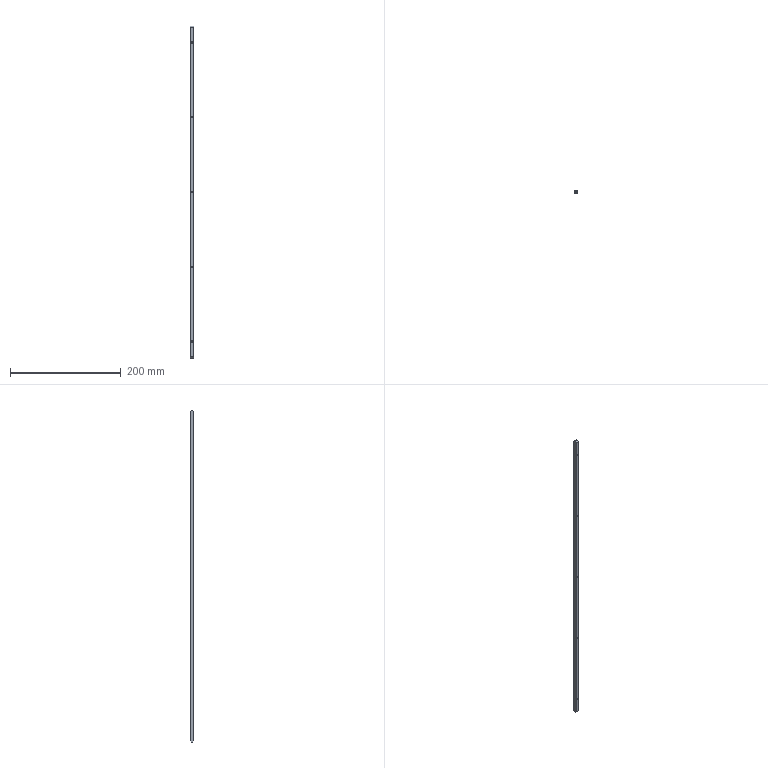Part | SolidWorks | features 3DProfileFeature 1, Chamfer 1, Extrusion 1, HoleWzd 1 | 1 solid | 20 faces | box 6 x 6 x 600 mm | volume 21405 mm3 | cylinder 10 | plane 10 | commonest cylinder face diameters 2.5 x10
STEP:
#1=CARTESIAN_POINT('',(0.,-3.,163.75));
#2=VERTEX_POINT('',#1);
#3=CARTESIAN_POINT('',(0.,-3.,166.25));
#4=VERTEX_POINT('',#3);
#5=CARTESIAN_POINT('',(0.,-3.,165.));
#6=DIRECTION('',(0.,1.,0.));
#7=DIRECTION('',(0.,0.,1.));
#8=AXIS2_PLACEMENT_3D('',#5,#6,#7);
#9=CIRCLE('',#8,1.25);
#10=EDGE_CURVE('',#2,#4,#9,.T.);
#11=ORIENTED_EDGE('',*,*,#10,.F.);
#12=CARTESIAN_POINT('',(0.,3.,163.75));
#13=VERTEX_POINT('',#12);
#14=CARTESIAN_POINT('',(0.,3.,163.75));
#15=DIRECTION('',(0.,1.,0.));
#16=VECTOR('',#15,1000.);
#17=LINE('',#14,#16);
#18=EDGE_CURVE('',#2,#13,#17,.T.);
#19=ORIENTED_EDGE('',*,*,#18,.T.);
#20=CARTESIAN_POINT('',(0.,3.,166.25));
#21=VERTEX_POINT('',#20);
#22=CARTESIAN_POINT('',(0.,3.,165.));
#23=DIRECTION('',(0.,1.,0.));
#24=DIRECTION('',(0.,0.,1.));
#25=AXIS2_PLACEMENT_3D('',#22,#23,#24);
#26=CIRCLE('',#25,1.25);
#27=EDGE_CURVE('',#13,#21,#26,.T.);
#28=ORIENTED_EDGE('',*,*,#27,.T.);
#29=CARTESIAN_POINT('',(0.,3.,166.25));
#30=DIRECTION('',(0.,1.,0.));
#31=VECTOR('',#30,1000.);
#32=LINE('',#29,#31);
#33=EDGE_CURVE('',#4,#21,#32,.T.);
#34=ORIENTED_EDGE('',*,*,#33,.F.);
#35=EDGE_LOOP('',(#11,#19,#28,#34));
#36=FACE_OUTER_BOUND('',#35,.T.);
#37=CARTESIAN_POINT('',(0.,3.,165.));
#38=DIRECTION('',(0.,1.,0.));
#39=DIRECTION('',(0.,0.,1.));
#40=AXIS2_PLACEMENT_3D('',#37,#38,#39);
#41=CYLINDRICAL_SURFACE('',#40,1.25);
#42=ADVANCED_FACE('',(#36),#41,.F.);
#43=CARTESIAN_POINT('',(0.,-3.,298.75));
#44=VERTEX_POINT('',#43);
#45=CARTESIAN_POINT('',(0.,-3.,301.25));
#46=VERTEX_POINT('',#45);
#47=CARTESIAN_POINT('',(0.,-3.,300.));
#48=DIRECTION('',(0.,1.,0.));
#49=DIRECTION('',(0.,0.,1.));
#50=AXIS2_PLACEMENT_3D('',#47,#48,#49);
#51=CIRCLE('',#50,1.25);
#52=EDGE_CURVE('',#44,#46,#51,.T.);
#53=ORIENTED_EDGE('',*,*,#52,.F.);
#54=CARTESIAN_POINT('',(0.,3.,298.75));
#55=VERTEX_POINT('',#54);
#56=CARTESIAN_POINT('',(0.,3.,298.75));
#57=DIRECTION('',(0.,1.,0.));
#58=VECTOR('',#57,1000.);
#59=LINE('',#56,#58);
#60=EDGE_CURVE('',#44,#55,#59,.T.);
#61=ORIENTED_EDGE('',*,*,#60,.T.);
#62=CARTESIAN_POINT('',(0.,3.,301.25));
#63=VERTEX_POINT('',#62);
#64=CARTESIAN_POINT('',(0.,3.,300.));
#65=DIRECTION('',(0.,1.,0.));
#66=DIRECTION('',(0.,0.,1.));
#67=AXIS2_PLACEMENT_3D('',#64,#65,#66);
#68=CIRCLE('',#67,1.25);
#69=EDGE_CURVE('',#55,#63,#68,.T.);
#70=ORIENTED_EDGE('',*,*,#69,.T.);
#71=CARTESIAN_POINT('',(0.,3.,301.25));
#72=DIRECTION('',(0.,1.,0.));
#73=VECTOR('',#72,1000.);
#74=LINE('',#71,#73);
#75=EDGE_CURVE('',#46,#63,#74,.T.);
#76=ORIENTED_EDGE('',*,*,#75,.F.);
#77=EDGE_LOOP('',(#53,#61,#70,#76));
#78=FACE_OUTER_BOUND('',#77,.T.);
#79=CARTESIAN_POINT('',(0.,3.,300.));
#80=DIRECTION('',(0.,1.,0.));
#81=DIRECTION('',(0.,0.,1.));
#82=AXIS2_PLACEMENT_3D('',#79,#80,#81);
#83=CYLINDRICAL_SURFACE('',#82,1.25);
#84=ADVANCED_FACE('',(#78),#83,.F.);
#85=CARTESIAN_POINT('',(0.,-3.,433.75));
#86=VERTEX_POINT('',#85);
#87=CARTESIAN_POINT('',(0.,-3.,436.25));
#88=VERTEX_POINT('',#87);
#89=CARTESIAN_POINT('',(0.,-3.,435.));
#90=DIRECTION('',(0.,1.,0.));
#91=DIRECTION('',(0.,0.,1.));
#92=AXIS2_PLACEMENT_3D('',#89,#90,#91);
#93=CIRCLE('',#92,1.25);
#94=EDGE_CURVE('',#86,#88,#93,.T.);
#95=ORIENTED_EDGE('',*,*,#94,.F.);
#96=CARTESIAN_POINT('',(0.,3.,433.75));
#97=VERTEX_POINT('',#96);
#98=CARTESIAN_POINT('',(0.,3.,433.75));
#99=DIRECTION('',(0.,1.,0.));
#100=VECTOR('',#99,1000.);
#101=LINE('',#98,#100);
#102=EDGE_CURVE('',#86,#97,#101,.T.);
#103=ORIENTED_EDGE('',*,*,#102,.T.);
#104=CARTESIAN_POINT('',(0.,3.,436.25));
#105=VERTEX_POINT('',#104);
#106=CARTESIAN_POINT('',(0.,3.,435.));
#107=DIRECTION('',(0.,1.,0.));
#108=DIRECTION('',(0.,0.,1.));
#109=AXIS2_PLACEMENT_3D('',#106,#107,#108);
#110=CIRCLE('',#109,1.25);
#111=EDGE_CURVE('',#97,#105,#110,.T.);
#112=ORIENTED_EDGE('',*,*,#111,.T.);
#113=CARTESIAN_POINT('',(0.,3.,436.25));
#114=DIRECTION('',(0.,1.,0.));
#115=VECTOR('',#114,1000.);
#116=LINE('',#113,#115);
#117=EDGE_CURVE('',#88,#105,#116,.T.);
#118=ORIENTED_EDGE('',*,*,#117,.F.);
#119=EDGE_LOOP('',(#95,#103,#112,#118));
#120=FACE_OUTER_BOUND('',#119,.T.);
#121=CARTESIAN_POINT('',(0.,3.,435.));
#122=DIRECTION('',(0.,1.,0.));
#123=DIRECTION('',(0.,0.,1.));
#124=AXIS2_PLACEMENT_3D('',#121,#122,#123);
#125=CYLINDRICAL_SURFACE('',#124,1.25);
#126=ADVANCED_FACE('',(#120),#125,.F.);
#127=CARTESIAN_POINT('',(0.,-3.,568.75));
#128=VERTEX_POINT('',#127);
#129=CARTESIAN_POINT('',(0.,-3.,571.25));
#130=VERTEX_POINT('',#129);
#131=CARTESIAN_POINT('',(0.,-3.,570.));
#132=DIRECTION('',(0.,1.,0.));
#133=DIRECTION('',(0.,0.,1.));
#134=AXIS2_PLACEMENT_3D('',#131,#132,#133);
#135=CIRCLE('',#134,1.25);
#136=EDGE_CURVE('',#128,#130,#135,.T.);
#137=ORIENTED_EDGE('',*,*,#136,.F.);
#138=CARTESIAN_POINT('',(0.,3.,568.75));
#139=VERTEX_POINT('',#138);
#140=CARTESIAN_POINT('',(0.,3.,568.75));
#141=DIRECTION('',(0.,1.,0.));
#142=VECTOR('',#141,1000.);
#143=LINE('',#140,#142);
#144=EDGE_CURVE('',#128,#139,#143,.T.);
#145=ORIENTED_EDGE('',*,*,#144,.T.);
#146=CARTESIAN_POINT('',(0.,3.,571.25));
#147=VERTEX_POINT('',#146);
#148=CARTESIAN_POINT('',(0.,3.,570.));
#149=DIRECTION('',(0.,1.,0.));
#150=DIRECTION('',(0.,0.,1.));
#151=AXIS2_PLACEMENT_3D('',#148,#149,#150);
#152=CIRCLE('',#151,1.25);
#153=EDGE_CURVE('',#139,#147,#152,.T.);
#154=ORIENTED_EDGE('',*,*,#153,.T.);
#155=CARTESIAN_POINT('',(0.,3.,571.25));
#156=DIRECTION('',(0.,1.,0.));
#157=VECTOR('',#156,1000.);
#158=LINE('',#155,#157);
#159=EDGE_CURVE('',#130,#147,#158,.T.);
#160=ORIENTED_EDGE('',*,*,#159,.F.);
#161=EDGE_LOOP('',(#137,#145,#154,#160));
#162=FACE_OUTER_BOUND('',#161,.T.);
#163=CARTESIAN_POINT('',(0.,3.,570.));
#164=DIRECTION('',(0.,1.,0.));
#165=DIRECTION('',(0.,0.,1.));
#166=AXIS2_PLACEMENT_3D('',#163,#164,#165);
#167=CYLINDRICAL_SURFACE('',#166,1.25);
#168=ADVANCED_FACE('',(#162),#167,.F.);
#169=CARTESIAN_POINT('',(0.,-3.,28.75));
#170=VERTEX_POINT('',#169);
#171=CARTESIAN_POINT('',(0.,-3.,31.25));
#172=VERTEX_POINT('',#171);
#173=CARTESIAN_POINT('',(0.,-3.,30.));
#174=DIRECTION('',(0.,1.,0.));
#175=DIRECTION('',(0.,0.,1.));
#176=AXIS2_PLACEMENT_3D('',#173,#174,#175);
#177=CIRCLE('',#176,1.25);
#178=EDGE_CURVE('',#170,#172,#177,.T.);
#179=ORIENTED_EDGE('',*,*,#178,.F.);
#180=CARTESIAN_POINT('',(0.,3.,28.75));
#181=VERTEX_POINT('',#180);
#182=CARTESIAN_POINT('',(0.,3.,28.75));
#183=DIRECTION('',(0.,1.,0.));
#184=VECTOR('',#183,1000.);
#185=LINE('',#182,#184);
#186=EDGE_CURVE('',#170,#181,#185,.T.);
#187=ORIENTED_EDGE('',*,*,#186,.T.);
#188=CARTESIAN_POINT('',(0.,3.,31.25));
#189=VERTEX_POINT('',#188);
#190=CARTESIAN_POINT('',(0.,3.,30.));
#191=DIRECTION('',(0.,1.,0.));
#192=DIRECTION('',(0.,0.,1.));
#193=AXIS2_PLACEMENT_3D('',#190,#191,#192);
#194=CIRCLE('',#193,1.25);
#195=EDGE_CURVE('',#181,#189,#194,.T.);
#196=ORIENTED_EDGE('',*,*,#195,.T.);
#197=CARTESIAN_POINT('',(0.,3.,31.25));
#198=DIRECTION('',(0.,1.,0.));
#199=VECTOR('',#198,1000.);
#200=LINE('',#197,#199);
#201=EDGE_CURVE('',#172,#189,#200,.T.);
#202=ORIENTED_EDGE('',*,*,#201,.F.);
#203=EDGE_LOOP('',(#179,#187,#196,#202));
#204=FACE_OUTER_BOUND('',#203,.T.);
#205=CARTESIAN_POINT('',(0.,3.,30.));
#206=DIRECTION('',(0.,1.,0.));
#207=DIRECTION('',(0.,0.,1.));
#208=AXIS2_PLACEMENT_3D('',#205,#206,#207);
#209=CYLINDRICAL_SURFACE('',#208,1.25);
#210=ADVANCED_FACE('',(#204),#209,.F.);
#211=CARTESIAN_POINT('',(3.,-3.,598.));
#212=VERTEX_POINT('',#211);
#213=CARTESIAN_POINT('',(3.,-3.,2.));
#214=VERTEX_POINT('',#213);
#215=CARTESIAN_POINT('',(3.,-3.,600.));
#216=DIRECTION('',(0.,0.,-1.));
#217=VECTOR('',#216,1000.);
#218=LINE('',#215,#217);
#219=EDGE_CURVE('',#212,#214,#218,.T.);
#220=ORIENTED_EDGE('',*,*,#219,.T.);
#221=CARTESIAN_POINT('',(3.,-1.,0.));
#222=VERTEX_POINT('',#221);
#223=CARTESIAN_POINT('',(3.,-3.,2.));
#224=DIRECTION('',(0.,0.7071,-0.7071));
#225=VECTOR('',#224,1000.);
#226=LINE('',#223,#225);
#227=EDGE_CURVE('',#214,#222,#226,.T.);
#228=ORIENTED_EDGE('',*,*,#227,.T.);
#229=CARTESIAN_POINT('',(3.,1.,0.));
#230=VERTEX_POINT('',#229);
#231=CARTESIAN_POINT('',(3.,3.,0.));
#232=DIRECTION('',(0.,1.,0.));
#233=VECTOR('',#232,1000.);
#234=LINE('',#231,#233);
#235=EDGE_CURVE('',#222,#230,#234,.T.);
#236=ORIENTED_EDGE('',*,*,#235,.T.);
#237=CARTESIAN_POINT('',(3.,3.,2.));
#238=VERTEX_POINT('',#237);
#239=CARTESIAN_POINT('',(3.,3.,2.));
#240=DIRECTION('',(0.,0.7071,0.7071));
#241=VECTOR('',#240,1000.);
#242=LINE('',#239,#241);
#243=EDGE_CURVE('',#230,#238,#242,.T.);
#244=ORIENTED_EDGE('',*,*,#243,.T.);
#245=CARTESIAN_POINT('',(3.,3.,598.));
#246=VERTEX_POINT('',#245);
#247=CARTESIAN_POINT('',(3.,3.,600.));
#248=DIRECTION('',(0.,0.,-1.));
#249=VECTOR('',#248,1000.);
#250=LINE('',#247,#249);
#251=EDGE_CURVE('',#246,#238,#250,.T.);
#252=ORIENTED_EDGE('',*,*,#251,.F.);
#253=CARTESIAN_POINT('',(3.,1.,600.));
#254=VERTEX_POINT('',#253);
#255=CARTESIAN_POINT('',(3.,1.,600.));
#256=DIRECTION('',(0.,-0.7071,0.7071));
#257=VECTOR('',#256,1000.);
#258=LINE('',#255,#257);
#259=EDGE_CURVE('',#246,#254,#258,.T.);
#260=ORIENTED_EDGE('',*,*,#259,.T.);
#261=CARTESIAN_POINT('',(3.,-1.,600.));
#262=VERTEX_POINT('',#261);
#263=CARTESIAN_POINT('',(3.,3.,600.));
#264=DIRECTION('',(0.,1.,0.));
#265=VECTOR('',#264,1000.);
#266=LINE('',#263,#265);
#267=EDGE_CURVE('',#262,#254,#266,.T.);
#268=ORIENTED_EDGE('',*,*,#267,.F.);
#269=CARTESIAN_POINT('',(3.,-1.,600.));
#270=DIRECTION('',(0.,-0.7071,-0.7071));
#271=VECTOR('',#270,1000.);
#272=LINE('',#269,#271);
#273=EDGE_CURVE('',#262,#212,#272,.T.);
#274=ORIENTED_EDGE('',*,*,#273,.T.);
#275=EDGE_LOOP('',(#220,#228,#236,#244,#252,#260,#268,#274));
#276=FACE_OUTER_BOUND('',#275,.T.);
#277=CARTESIAN_POINT('',(3.,3.,600.));
#278=DIRECTION('',(-1.,0.,0.));
#279=DIRECTION('',(0.,-1.,0.));
#280=AXIS2_PLACEMENT_3D('',#277,#278,#279);
#281=PLANE('',#280);
#282=ADVANCED_FACE('',(#276),#281,.F.);
#283=CARTESIAN_POINT('',(0.,3.,165.));
#284=DIRECTION('',(0.,1.,0.));
#285=DIRECTION('',(0.,0.,1.));
#286=AXIS2_PLACEMENT_3D('',#283,#284,#285);
#287=CIRCLE('',#286,1.25);
#288=EDGE_CURVE('',#21,#13,#287,.T.);
#289=ORIENTED_EDGE('',*,*,#288,.F.);
#290=ORIENTED_EDGE('',*,*,#27,.F.);
#291=EDGE_LOOP('',(#289,#290));
#292=FACE_BOUND('',#291,.T.);
#293=CARTESIAN_POINT('',(0.,3.,300.));
#294=DIRECTION('',(0.,1.,0.));
#295=DIRECTION('',(0.,0.,1.));
#296=AXIS2_PLACEMENT_3D('',#293,#294,#295);
#297=CIRCLE('',#296,1.25);
#298=EDGE_CURVE('',#63,#55,#297,.T.);
#299=ORIENTED_EDGE('',*,*,#298,.F.);
#300=ORIENTED_EDGE('',*,*,#69,.F.);
#301=EDGE_LOOP('',(#299,#300));
#302=FACE_BOUND('',#301,.T.);
#303=CARTESIAN_POINT('',(0.,3.,435.));
#304=DIRECTION('',(0.,1.,0.));
#305=DIRECTION('',(0.,0.,1.));
#306=AXIS2_PLACEMENT_3D('',#303,#304,#305);
#307=CIRCLE('',#306,1.25);
#308=EDGE_CURVE('',#105,#97,#307,.T.);
#309=ORIENTED_EDGE('',*,*,#308,.F.);
#310=ORIENTED_EDGE('',*,*,#111,.F.);
#311=EDGE_LOOP('',(#309,#310));
#312=FACE_BOUND('',#311,.T.);
#313=CARTESIAN_POINT('',(0.,3.,570.));
#314=DIRECTION('',(0.,1.,0.));
#315=DIRECTION('',(0.,0.,1.));
#316=AXIS2_PLACEMENT_3D('',#313,#314,#315);
#317=CIRCLE('',#316,1.25);
#318=EDGE_CURVE('',#147,#139,#317,.T.);
#319=ORIENTED_EDGE('',*,*,#318,.F.);
#320=ORIENTED_EDGE('',*,*,#153,.F.);
#321=EDGE_LOOP('',(#319,#320));
#322=FACE_BOUND('',#321,.T.);
#323=CARTESIAN_POINT('',(0.,3.,30.));
#324=DIRECTION('',(0.,1.,0.));
#325=DIRECTION('',(0.,0.,1.));
#326=AXIS2_PLACEMENT_3D('',#323,#324,#325);
#327=CIRCLE('',#326,1.25);
#328=EDGE_CURVE('',#189,#181,#327,.T.);
#329=ORIENTED_EDGE('',*,*,#328,.F.);
#330=ORIENTED_EDGE('',*,*,#195,.F.);
#331=EDGE_LOOP('',(#329,#330));
#332=FACE_BOUND('',#331,.T.);
#333=ORIENTED_EDGE('',*,*,#251,.T.);
#334=CARTESIAN_POINT('',(-3.,3.,2.));
#335=VERTEX_POINT('',#334);
#336=CARTESIAN_POINT('',(-3.,3.,2.));
#337=DIRECTION('',(-1.,0.,0.));
#338=VECTOR('',#337,1000.);
#339=LINE('',#336,#338);
#340=EDGE_CURVE('',#238,#335,#339,.T.);
#341=ORIENTED_EDGE('',*,*,#340,.T.);
#342=CARTESIAN_POINT('',(-3.,3.,598.));
#343=VERTEX_POINT('',#342);
#344=CARTESIAN_POINT('',(-3.,3.,600.));
#345=DIRECTION('',(0.,0.,-1.));
#346=VECTOR('',#345,1000.);
#347=LINE('',#344,#346);
#348=EDGE_CURVE('',#343,#335,#347,.T.);
#349=ORIENTED_EDGE('',*,*,#348,.F.);
#350=CARTESIAN_POINT('',(3.,3.,598.));
#351=DIRECTION('',(1.,0.,0.));
#352=VECTOR('',#351,1000.);
#353=LINE('',#350,#352);
#354=EDGE_CURVE('',#343,#246,#353,.T.);
#355=ORIENTED_EDGE('',*,*,#354,.T.);
#356=EDGE_LOOP('',(#333,#341,#349,#355));
#357=FACE_OUTER_BOUND('',#356,.T.);
#358=CARTESIAN_POINT('',(-3.,3.,600.));
#359=DIRECTION('',(0.,-1.,0.));
#360=DIRECTION('',(0.,0.,-1.));
#361=AXIS2_PLACEMENT_3D('',#358,#359,#360);
#362=PLANE('',#361);
#363=ADVANCED_FACE('',(#292,#302,#312,#322,#332,#357),#362,.F.);
#364=CARTESIAN_POINT('',(-3.,1.,0.));
#365=VERTEX_POINT('',#364);
#366=CARTESIAN_POINT('',(-3.,-1.,0.));
#367=VERTEX_POINT('',#366);
#368=CARTESIAN_POINT('',(-3.,3.,0.));
#369=DIRECTION('',(0.,-1.,0.));
#370=VECTOR('',#369,1000.);
#371=LINE('',#368,#370);
#372=EDGE_CURVE('',#365,#367,#371,.T.);
#373=ORIENTED_EDGE('',*,*,#372,.T.);
#374=CARTESIAN_POINT('',(-3.,-3.,2.));
#375=VERTEX_POINT('',#374);
#376=CARTESIAN_POINT('',(-3.,-3.,2.));
#377=DIRECTION('',(0.,-0.7071,0.7071));
#378=VECTOR('',#377,1000.);
#379=LINE('',#376,#378);
#380=EDGE_CURVE('',#367,#375,#379,.T.);
#381=ORIENTED_EDGE('',*,*,#380,.T.);
#382=CARTESIAN_POINT('',(-3.,-3.,598.));
#383=VERTEX_POINT('',#382);
#384=CARTESIAN_POINT('',(-3.,-3.,600.));
#385=DIRECTION('',(0.,0.,-1.));
#386=VECTOR('',#385,1000.);
#387=LINE('',#384,#386);
#388=EDGE_CURVE('',#383,#375,#387,.T.);
#389=ORIENTED_EDGE('',*,*,#388,.F.);
#390=CARTESIAN_POINT('',(-3.,-1.,600.));
#391=VERTEX_POINT('',#390);
#392=CARTESIAN_POINT('',(-3.,-1.,600.));
#393=DIRECTION('',(0.,0.7071,0.7071));
#394=VECTOR('',#393,1000.);
#395=LINE('',#392,#394);
#396=EDGE_CURVE('',#383,#391,#395,.T.);
#397=ORIENTED_EDGE('',*,*,#396,.T.);
#398=CARTESIAN_POINT('',(-3.,1.,600.));
#399=VERTEX_POINT('',#398);
#400=CARTESIAN_POINT('',(-3.,3.,600.));
#401=DIRECTION('',(0.,-1.,0.));
#402=VECTOR('',#401,1000.);
#403=LINE('',#400,#402);
#404=EDGE_CURVE('',#399,#391,#403,.T.);
#405=ORIENTED_EDGE('',*,*,#404,.F.);
#406=CARTESIAN_POINT('',(-3.,1.,600.));
#407=DIRECTION('',(0.,0.7071,-0.7071));
#408=VECTOR('',#407,1000.);
#409=LINE('',#406,#408);
#410=EDGE_CURVE('',#399,#343,#409,.T.);
#411=ORIENTED_EDGE('',*,*,#410,.T.);
#412=ORIENTED_EDGE('',*,*,#348,.T.);
#413=CARTESIAN_POINT('',(-3.,3.,2.));
#414=DIRECTION('',(0.,-0.7071,-0.7071));
#415=VECTOR('',#414,1000.);
#416=LINE('',#413,#415);
#417=EDGE_CURVE('',#335,#365,#416,.T.);
#418=ORIENTED_EDGE('',*,*,#417,.T.);
#419=EDGE_LOOP('',(#373,#381,#389,#397,#405,#411,#412,#418));
#420=FACE_OUTER_BOUND('',#419,.T.);
#421=CARTESIAN_POINT('',(-3.,3.,600.));
#422=DIRECTION('',(1.,0.,0.));
#423=DIRECTION('',(0.,1.,0.));
#424=AXIS2_PLACEMENT_3D('',#421,#422,#423);
#425=PLANE('',#424);
#426=ADVANCED_FACE('',(#420),#425,.F.);
#427=CARTESIAN_POINT('',(0.,-3.,165.));
#428=DIRECTION('',(0.,1.,0.));
#429=DIRECTION('',(0.,0.,1.));
#430=AXIS2_PLACEMENT_3D('',#427,#428,#429);
#431=CIRCLE('',#430,1.25);
#432=EDGE_CURVE('',#4,#2,#431,.T.);
#433=ORIENTED_EDGE('',*,*,#432,.T.);
#434=ORIENTED_EDGE('',*,*,#10,.T.);
#435=EDGE_LOOP('',(#433,#434));
#436=FACE_BOUND('',#435,.T.);
#437=CARTESIAN_POINT('',(0.,-3.,300.));
#438=DIRECTION('',(0.,1.,0.));
#439=DIRECTION('',(0.,0.,1.));
#440=AXIS2_PLACEMENT_3D('',#437,#438,#439);
#441=CIRCLE('',#440,1.25);
#442=EDGE_CURVE('',#46,#44,#441,.T.);
#443=ORIENTED_EDGE('',*,*,#442,.T.);
#444=ORIENTED_EDGE('',*,*,#52,.T.);
#445=EDGE_LOOP('',(#443,#444));
#446=FACE_BOUND('',#445,.T.);
#447=CARTESIAN_POINT('',(0.,-3.,435.));
#448=DIRECTION('',(0.,1.,0.));
#449=DIRECTION('',(0.,0.,1.));
#450=AXIS2_PLACEMENT_3D('',#447,#448,#449);
#451=CIRCLE('',#450,1.25);
#452=EDGE_CURVE('',#88,#86,#451,.T.);
#453=ORIENTED_EDGE('',*,*,#452,.T.);
#454=ORIENTED_EDGE('',*,*,#94,.T.);
#455=EDGE_LOOP('',(#453,#454));
#456=FACE_BOUND('',#455,.T.);
#457=CARTESIAN_POINT('',(0.,-3.,570.));
#458=DIRECTION('',(0.,1.,0.));
#459=DIRECTION('',(0.,0.,1.));
#460=AXIS2_PLACEMENT_3D('',#457,#458,#459);
#461=CIRCLE('',#460,1.25);
#462=EDGE_CURVE('',#130,#128,#461,.T.);
#463=ORIENTED_EDGE('',*,*,#462,.T.);
#464=ORIENTED_EDGE('',*,*,#136,.T.);
#465=EDGE_LOOP('',(#463,#464));
#466=FACE_BOUND('',#465,.T.);
#467=CARTESIAN_POINT('',(0.,-3.,30.));
#468=DIRECTION('',(0.,1.,0.));
#469=DIRECTION('',(0.,0.,1.));
#470=AXIS2_PLACEMENT_3D('',#467,#468,#469);
#471=CIRCLE('',#470,1.25);
#472=EDGE_CURVE('',#172,#170,#471,.T.);
#473=ORIENTED_EDGE('',*,*,#472,.T.);
#474=ORIENTED_EDGE('',*,*,#178,.T.);
#475=EDGE_LOOP('',(#473,#474));
#476=FACE_BOUND('',#475,.T.);
#477=ORIENTED_EDGE('',*,*,#388,.T.);
#478=CARTESIAN_POINT('',(-3.,-3.,2.));
#479=DIRECTION('',(1.,0.,0.));
#480=VECTOR('',#479,1000.);
#481=LINE('',#478,#480);
#482=EDGE_CURVE('',#375,#214,#481,.T.);
#483=ORIENTED_EDGE('',*,*,#482,.T.);
#484=ORIENTED_EDGE('',*,*,#219,.F.);
#485=CARTESIAN_POINT('',(-3.,-3.,598.));
#486=DIRECTION('',(-1.,0.,0.));
#487=VECTOR('',#486,1000.);
#488=LINE('',#485,#487);
#489=EDGE_CURVE('',#212,#383,#488,.T.);
#490=ORIENTED_EDGE('',*,*,#489,.T.);
#491=EDGE_LOOP('',(#477,#483,#484,#490));
#492=FACE_OUTER_BOUND('',#491,.T.);
#493=CARTESIAN_POINT('',(-3.,-3.,600.));
#494=DIRECTION('',(0.,1.,0.));
#495=DIRECTION('',(0.,0.,1.));
#496=AXIS2_PLACEMENT_3D('',#493,#494,#495);
#497=PLANE('',#496);
#498=ADVANCED_FACE('',(#436,#446,#456,#466,#476,#492),#497,.F.);
#499=ORIENTED_EDGE('',*,*,#404,.T.);
#500=CARTESIAN_POINT('',(3.,-1.,600.));
#501=DIRECTION('',(1.,0.,0.));
#502=VECTOR('',#501,1000.);
#503=LINE('',#500,#502);
#504=EDGE_CURVE('',#391,#262,#503,.T.);
#505=ORIENTED_EDGE('',*,*,#504,.T.);
#506=ORIENTED_EDGE('',*,*,#267,.T.);
#507=CARTESIAN_POINT('',(-3.,1.,600.));
#508=DIRECTION('',(-1.,0.,0.));
#509=VECTOR('',#508,1000.);
#510=LINE('',#507,#509);
#511=EDGE_CURVE('',#254,#399,#510,.T.);
#512=ORIENTED_EDGE('',*,*,#511,.T.);
#513=EDGE_LOOP('',(#499,#505,#506,#512));
#514=FACE_OUTER_BOUND('',#513,.T.);
#515=CARTESIAN_POINT('',(0.,0.,600.));
#516=DIRECTION('',(0.,0.,1.));
#517=DIRECTION('',(1.,0.,0.));
#518=AXIS2_PLACEMENT_3D('',#515,#516,#517);
#519=PLANE('',#518);
#520=ADVANCED_FACE('',(#514),#519,.T.);
#521=ORIENTED_EDGE('',*,*,#235,.F.);
#522=CARTESIAN_POINT('',(0.,-1.,0.));
#523=DIRECTION('',(-1.,0.,0.));
#524=VECTOR('',#523,1000.);
#525=LINE('',#522,#524);
#526=EDGE_CURVE('',#222,#367,#525,.T.);
#527=ORIENTED_EDGE('',*,*,#526,.T.);
#528=ORIENTED_EDGE('',*,*,#372,.F.);
#529=CARTESIAN_POINT('',(0.,1.,0.));
#530=DIRECTION('',(1.,0.,0.));
#531=VECTOR('',#530,1000.);
#532=LINE('',#529,#531);
#533=EDGE_CURVE('',#365,#230,#532,.T.);
#534=ORIENTED_EDGE('',*,*,#533,.T.);
#535=EDGE_LOOP('',(#521,#527,#528,#534));
#536=FACE_OUTER_BOUND('',#535,.T.);
#537=CARTESIAN_POINT('',(0.,0.,0.));
#538=DIRECTION('',(0.,0.,1.));
#539=DIRECTION('',(1.,0.,0.));
#540=AXIS2_PLACEMENT_3D('',#537,#538,#539);
#541=PLANE('',#540);
#542=ADVANCED_FACE('',(#536),#541,.F.);
#543=ORIENTED_EDGE('',*,*,#186,.F.);
#544=ORIENTED_EDGE('',*,*,#472,.F.);
#545=ORIENTED_EDGE('',*,*,#201,.T.);
#546=ORIENTED_EDGE('',*,*,#328,.T.);
#547=EDGE_LOOP('',(#543,#544,#545,#546));
#548=FACE_OUTER_BOUND('',#547,.T.);
#549=CARTESIAN_POINT('',(0.,3.,30.));
#550=DIRECTION('',(0.,1.,0.));
#551=DIRECTION('',(0.,0.,1.));
#552=AXIS2_PLACEMENT_3D('',#549,#550,#551);
#553=CYLINDRICAL_SURFACE('',#552,1.25);
#554=ADVANCED_FACE('',(#548),#553,.F.);
#555=ORIENTED_EDGE('',*,*,#144,.F.);
#556=ORIENTED_EDGE('',*,*,#462,.F.);
#557=ORIENTED_EDGE('',*,*,#159,.T.);
#558=ORIENTED_EDGE('',*,*,#318,.T.);
#559=EDGE_LOOP('',(#555,#556,#557,#558));
#560=FACE_OUTER_BOUND('',#559,.T.);
#561=CARTESIAN_POINT('',(0.,3.,570.));
#562=DIRECTION('',(0.,1.,0.));
#563=DIRECTION('',(0.,0.,1.));
#564=AXIS2_PLACEMENT_3D('',#561,#562,#563);
#565=CYLINDRICAL_SURFACE('',#564,1.25);
#566=ADVANCED_FACE('',(#560),#565,.F.);
#567=ORIENTED_EDGE('',*,*,#102,.F.);
#568=ORIENTED_EDGE('',*,*,#452,.F.);
#569=ORIENTED_EDGE('',*,*,#117,.T.);
#570=ORIENTED_EDGE('',*,*,#308,.T.);
#571=EDGE_LOOP('',(#567,#568,#569,#570));
#572=FACE_OUTER_BOUND('',#571,.T.);
#573=CARTESIAN_POINT('',(0.,3.,435.));
#574=DIRECTION('',(0.,1.,0.));
#575=DIRECTION('',(0.,0.,1.));
#576=AXIS2_PLACEMENT_3D('',#573,#574,#575);
#577=CYLINDRICAL_SURFACE('',#576,1.25);
#578=ADVANCED_FACE('',(#572),#577,.F.);
#579=ORIENTED_EDGE('',*,*,#60,.F.);
#580=ORIENTED_EDGE('',*,*,#442,.F.);
#581=ORIENTED_EDGE('',*,*,#75,.T.);
#582=ORIENTED_EDGE('',*,*,#298,.T.);
#583=EDGE_LOOP('',(#579,#580,#581,#582));
#584=FACE_OUTER_BOUND('',#583,.T.);
#585=CARTESIAN_POINT('',(0.,3.,300.));
#586=DIRECTION('',(0.,1.,0.));
#587=DIRECTION('',(0.,0.,1.));
#588=AXIS2_PLACEMENT_3D('',#585,#586,#587);
#589=CYLINDRICAL_SURFACE('',#588,1.25);
#590=ADVANCED_FACE('',(#584),#589,.F.);
#591=ORIENTED_EDGE('',*,*,#18,.F.);
#592=ORIENTED_EDGE('',*,*,#432,.F.);
#593=ORIENTED_EDGE('',*,*,#33,.T.);
#594=ORIENTED_EDGE('',*,*,#288,.T.);
#595=EDGE_LOOP('',(#591,#592,#593,#594));
#596=FACE_OUTER_BOUND('',#595,.T.);
#597=CARTESIAN_POINT('',(0.,3.,165.));
#598=DIRECTION('',(0.,1.,0.));
#599=DIRECTION('',(0.,0.,1.));
#600=AXIS2_PLACEMENT_3D('',#597,#598,#599);
#601=CYLINDRICAL_SURFACE('',#600,1.25);
#602=ADVANCED_FACE('',(#596),#601,.F.);
#603=ORIENTED_EDGE('',*,*,#380,.F.);
#604=ORIENTED_EDGE('',*,*,#526,.F.);
#605=ORIENTED_EDGE('',*,*,#227,.F.);
#606=ORIENTED_EDGE('',*,*,#482,.F.);
#607=EDGE_LOOP('',(#603,#604,#605,#606));
#608=FACE_OUTER_BOUND('',#607,.T.);
#609=CARTESIAN_POINT('',(-3.,-3.,2.));
#610=DIRECTION('',(0.,0.7071,0.7071));
#611=DIRECTION('',(1.,0.,0.));
#612=AXIS2_PLACEMENT_3D('',#609,#610,#611);
#613=PLANE('',#612);
#614=ADVANCED_FACE('',(#608),#613,.F.);
#615=ORIENTED_EDGE('',*,*,#243,.F.);
#616=ORIENTED_EDGE('',*,*,#533,.F.);
#617=ORIENTED_EDGE('',*,*,#417,.F.);
#618=ORIENTED_EDGE('',*,*,#340,.F.);
#619=EDGE_LOOP('',(#615,#616,#617,#618));
#620=FACE_OUTER_BOUND('',#619,.T.);
#621=CARTESIAN_POINT('',(-3.,3.,2.));
#622=DIRECTION('',(0.,-0.7071,0.7071));
#623=DIRECTION('',(-1.,0.,0.));
#624=AXIS2_PLACEMENT_3D('',#621,#622,#623);
#625=PLANE('',#624);
#626=ADVANCED_FACE('',(#620),#625,.F.);
#627=ORIENTED_EDGE('',*,*,#396,.F.);
#628=ORIENTED_EDGE('',*,*,#489,.F.);
#629=ORIENTED_EDGE('',*,*,#273,.F.);
#630=ORIENTED_EDGE('',*,*,#504,.F.);
#631=EDGE_LOOP('',(#627,#628,#629,#630));
#632=FACE_OUTER_BOUND('',#631,.T.);
#633=CARTESIAN_POINT('',(0.,-1.,600.));
#634=DIRECTION('',(0.,-0.7071,0.7071));
#635=DIRECTION('',(-1.,0.,0.));
#636=AXIS2_PLACEMENT_3D('',#633,#634,#635);
#637=PLANE('',#636);
#638=ADVANCED_FACE('',(#632),#637,.T.);
#639=ORIENTED_EDGE('',*,*,#259,.F.);
#640=ORIENTED_EDGE('',*,*,#354,.F.);
#641=ORIENTED_EDGE('',*,*,#410,.F.);
#642=ORIENTED_EDGE('',*,*,#511,.F.);
#643=EDGE_LOOP('',(#639,#640,#641,#642));
#644=FACE_OUTER_BOUND('',#643,.T.);
#645=CARTESIAN_POINT('',(0.,1.,600.));
#646=DIRECTION('',(0.,0.7071,0.7071));
#647=DIRECTION('',(1.,0.,0.));
#648=AXIS2_PLACEMENT_3D('',#645,#646,#647);
#649=PLANE('',#648);
#650=ADVANCED_FACE('',(#644),#649,.T.);
#651=CLOSED_SHELL('',(#42,#84,#126,#168,#210,#282,#363,#426,#498,#520,#542,#554,#566,#578,#590,#602,#614,#626,#638,#650));
#652=MANIFOLD_SOLID_BREP('',#651);
#653=CARTESIAN_POINT('',(0.,0.,0.));
#654=DIRECTION('',(0.,0.,1.));
#655=DIRECTION('',(1.,0.,0.));
#656=AXIS2_PLACEMENT_3D('',#653,#654,#655);
#657=(LENGTH_UNIT()NAMED_UNIT(*)SI_UNIT(.MILLI.,.METRE.));
#658=UNCERTAINTY_MEASURE_WITH_UNIT(LENGTH_MEASURE(0.00001),#657,'','');
#659=(NAMED_UNIT(*)PLANE_ANGLE_UNIT()SI_UNIT($,.RADIAN.));
#660=(NAMED_UNIT(*)SI_UNIT($,.STERADIAN.)SOLID_ANGLE_UNIT());
#661=(GEOMETRIC_REPRESENTATION_CONTEXT(3)GLOBAL_UNCERTAINTY_ASSIGNED_CONTEXT((#658))GLOBAL_UNIT_ASSIGNED_CONTEXT((#657,#659,#660))REPRESENTATION_CONTEXT('',''));
#662=ADVANCED_BREP_SHAPE_REPRESENTATION('',(#652,#656),#661);